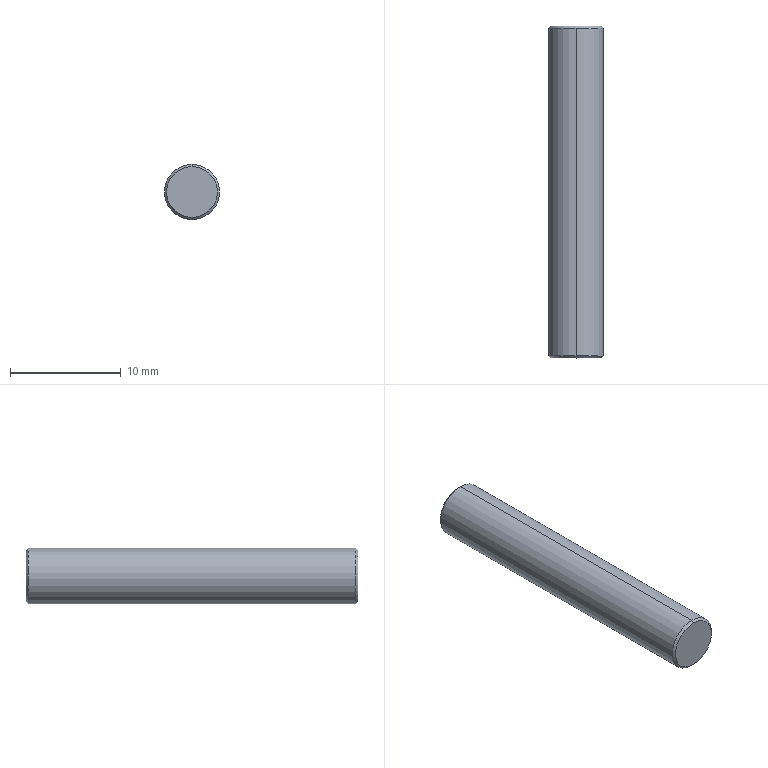Part | STEP file | 06-01-11 fibre mounting seat | 1 solid | 12 faces | box 5 x 30 x 5 mm | volume 550.393 mm3 | cone 6 | cylinder 4 | plane 2 | commonest cylinder face diameters 2.5 x2 5 x2
STEP:
#1=CARTESIAN_POINT('',(0.,22.5,-1.25));
#2=VERTEX_POINT('',#1);
#3=CARTESIAN_POINT('',(0.,22.5,1.25));
#4=VERTEX_POINT('',#3);
#5=CARTESIAN_POINT('',(0.,22.5,0.));
#6=DIRECTION('',(0.,1.,0.));
#7=DIRECTION('',(0.,0.,1.));
#8=AXIS2_PLACEMENT_3D('',#5,#6,#7);
#9=CIRCLE('',#8,1.25);
#10=EDGE_CURVE('',#2,#4,#9,.T.);
#11=ORIENTED_EDGE('',*,*,#10,.F.);
#12=CARTESIAN_POINT('',(0.,30.,-1.25));
#13=VERTEX_POINT('',#12);
#14=CARTESIAN_POINT('',(0.,30.,-1.25));
#15=DIRECTION('',(0.,1.,0.));
#16=VECTOR('',#15,1000.);
#17=LINE('',#14,#16);
#18=EDGE_CURVE('',#2,#13,#17,.T.);
#19=ORIENTED_EDGE('',*,*,#18,.T.);
#20=CARTESIAN_POINT('',(0.,30.,1.25));
#21=VERTEX_POINT('',#20);
#22=CARTESIAN_POINT('',(0.,30.,0.));
#23=DIRECTION('',(0.,1.,0.));
#24=DIRECTION('',(0.,0.,1.));
#25=AXIS2_PLACEMENT_3D('',#22,#23,#24);
#26=CIRCLE('',#25,1.25);
#27=EDGE_CURVE('',#13,#21,#26,.T.);
#28=ORIENTED_EDGE('',*,*,#27,.T.);
#29=CARTESIAN_POINT('',(0.,30.,1.25));
#30=DIRECTION('',(0.,1.,0.));
#31=VECTOR('',#30,1000.);
#32=LINE('',#29,#31);
#33=EDGE_CURVE('',#4,#21,#32,.T.);
#34=ORIENTED_EDGE('',*,*,#33,.F.);
#35=EDGE_LOOP('',(#11,#19,#28,#34));
#36=FACE_OUTER_BOUND('',#35,.T.);
#37=CARTESIAN_POINT('',(0.,30.,0.));
#38=DIRECTION('',(0.,1.,0.));
#39=DIRECTION('',(0.,0.,1.));
#40=AXIS2_PLACEMENT_3D('',#37,#38,#39);
#41=CYLINDRICAL_SURFACE('',#40,1.25);
#42=ADVANCED_FACE('',(#36),#41,.F.);
#43=CARTESIAN_POINT('',(0.,21.749,0.));
#44=VERTEX_POINT('',#43);
#45=CARTESIAN_POINT('',(0.,22.5,1.25));
#46=DIRECTION('',(0.,0.515,0.8572));
#47=VECTOR('',#46,1000.);
#48=LINE('',#45,#47);
#49=EDGE_CURVE('',#44,#4,#48,.T.);
#50=ORIENTED_EDGE('',*,*,#49,.F.);
#51=CARTESIAN_POINT('',(0.,22.5,-1.25));
#52=DIRECTION('',(0.,0.515,-0.8572));
#53=VECTOR('',#52,1000.);
#54=LINE('',#51,#53);
#55=EDGE_CURVE('',#44,#2,#54,.T.);
#56=ORIENTED_EDGE('',*,*,#55,.T.);
#57=ORIENTED_EDGE('',*,*,#10,.T.);
#58=EDGE_LOOP('',(#50,#56,#57));
#59=FACE_OUTER_BOUND('',#58,.T.);
#60=CARTESIAN_POINT('',(0.,22.5,0.));
#61=DIRECTION('',(0.,1.,0.));
#62=DIRECTION('',(0.,0.,1.));
#63=AXIS2_PLACEMENT_3D('',#60,#61,#62);
#64=CONICAL_SURFACE('',#63,1.25,1.03);
#65=ADVANCED_FACE('',(#59),#64,.F.);
#66=CARTESIAN_POINT('',(0.,30.,2.3));
#67=VERTEX_POINT('',#66);
#68=CARTESIAN_POINT('',(0.,30.,-2.3));
#69=VERTEX_POINT('',#68);
#70=CARTESIAN_POINT('',(0.,30.,0.));
#71=DIRECTION('',(0.,1.,0.));
#72=DIRECTION('',(0.,0.,1.));
#73=AXIS2_PLACEMENT_3D('',#70,#71,#72);
#74=CIRCLE('',#73,2.3);
#75=EDGE_CURVE('',#67,#69,#74,.T.);
#76=ORIENTED_EDGE('',*,*,#75,.F.);
#77=CARTESIAN_POINT('',(0.,29.8,2.5));
#78=VERTEX_POINT('',#77);
#79=CARTESIAN_POINT('',(0.,30.,2.3));
#80=DIRECTION('',(0.,-0.7071,0.7071));
#81=VECTOR('',#80,1000.);
#82=LINE('',#79,#81);
#83=EDGE_CURVE('',#67,#78,#82,.T.);
#84=ORIENTED_EDGE('',*,*,#83,.T.);
#85=CARTESIAN_POINT('',(0.,29.8,-2.5));
#86=VERTEX_POINT('',#85);
#87=CARTESIAN_POINT('',(0.,29.8,0.));
#88=DIRECTION('',(0.,-1.,0.));
#89=DIRECTION('',(0.,0.,1.));
#90=AXIS2_PLACEMENT_3D('',#87,#88,#89);
#91=CIRCLE('',#90,2.5);
#92=EDGE_CURVE('',#86,#78,#91,.T.);
#93=ORIENTED_EDGE('',*,*,#92,.F.);
#94=CARTESIAN_POINT('',(0.,30.,-2.3));
#95=DIRECTION('',(0.,-0.7071,-0.7071));
#96=VECTOR('',#95,1000.);
#97=LINE('',#94,#96);
#98=EDGE_CURVE('',#69,#86,#97,.T.);
#99=ORIENTED_EDGE('',*,*,#98,.F.);
#100=EDGE_LOOP('',(#76,#84,#93,#99));
#101=FACE_OUTER_BOUND('',#100,.T.);
#102=CARTESIAN_POINT('',(0.,30.,0.));
#103=DIRECTION('',(0.,-1.,0.));
#104=DIRECTION('',(0.,0.,-1.));
#105=AXIS2_PLACEMENT_3D('',#102,#103,#104);
#106=CONICAL_SURFACE('',#105,2.3,0.7854);
#107=ADVANCED_FACE('',(#101),#106,.T.);
#108=CARTESIAN_POINT('',(0.,0.,-2.3));
#109=VERTEX_POINT('',#108);
#110=CARTESIAN_POINT('',(0.,0.,2.3));
#111=VERTEX_POINT('',#110);
#112=CARTESIAN_POINT('',(0.,0.,0.));
#113=DIRECTION('',(0.,-1.,0.));
#114=DIRECTION('',(0.,0.,1.));
#115=AXIS2_PLACEMENT_3D('',#112,#113,#114);
#116=CIRCLE('',#115,2.3);
#117=EDGE_CURVE('',#109,#111,#116,.T.);
#118=ORIENTED_EDGE('',*,*,#117,.F.);
#119=CARTESIAN_POINT('',(0.,0.2,-2.5));
#120=VERTEX_POINT('',#119);
#121=CARTESIAN_POINT('',(0.,0.2,-2.5));
#122=DIRECTION('',(0.,0.7071,-0.7071));
#123=VECTOR('',#122,1000.);
#124=LINE('',#121,#123);
#125=EDGE_CURVE('',#109,#120,#124,.T.);
#126=ORIENTED_EDGE('',*,*,#125,.T.);
#127=CARTESIAN_POINT('',(0.,0.2,2.5));
#128=VERTEX_POINT('',#127);
#129=CARTESIAN_POINT('',(0.,0.2,0.));
#130=DIRECTION('',(0.,1.,0.));
#131=DIRECTION('',(0.,0.,1.));
#132=AXIS2_PLACEMENT_3D('',#129,#130,#131);
#133=CIRCLE('',#132,2.5);
#134=EDGE_CURVE('',#128,#120,#133,.T.);
#135=ORIENTED_EDGE('',*,*,#134,.F.);
#136=CARTESIAN_POINT('',(0.,0.2,2.5));
#137=DIRECTION('',(0.,0.7071,0.7071));
#138=VECTOR('',#137,1000.);
#139=LINE('',#136,#138);
#140=EDGE_CURVE('',#111,#128,#139,.T.);
#141=ORIENTED_EDGE('',*,*,#140,.F.);
#142=EDGE_LOOP('',(#118,#126,#135,#141));
#143=FACE_OUTER_BOUND('',#142,.T.);
#144=CARTESIAN_POINT('',(0.,0.2,0.));
#145=DIRECTION('',(0.,1.,0.));
#146=DIRECTION('',(0.,0.,1.));
#147=AXIS2_PLACEMENT_3D('',#144,#145,#146);
#148=CONICAL_SURFACE('',#147,2.5,0.7854);
#149=ADVANCED_FACE('',(#143),#148,.T.);
#150=ORIENTED_EDGE('',*,*,#92,.T.);
#151=CARTESIAN_POINT('',(0.,30.,2.5));
#152=DIRECTION('',(0.,-1.,0.));
#153=VECTOR('',#152,1000.);
#154=LINE('',#151,#153);
#155=EDGE_CURVE('',#78,#128,#154,.T.);
#156=ORIENTED_EDGE('',*,*,#155,.T.);
#157=ORIENTED_EDGE('',*,*,#134,.T.);
#158=CARTESIAN_POINT('',(0.,30.,-2.5));
#159=DIRECTION('',(0.,-1.,0.));
#160=VECTOR('',#159,1000.);
#161=LINE('',#158,#160);
#162=EDGE_CURVE('',#86,#120,#161,.T.);
#163=ORIENTED_EDGE('',*,*,#162,.F.);
#164=EDGE_LOOP('',(#150,#156,#157,#163));
#165=FACE_OUTER_BOUND('',#164,.T.);
#166=CARTESIAN_POINT('',(0.,30.,0.));
#167=DIRECTION('',(0.,-1.,0.));
#168=DIRECTION('',(0.,0.,-1.));
#169=AXIS2_PLACEMENT_3D('',#166,#167,#168);
#170=CYLINDRICAL_SURFACE('',#169,2.5);
#171=ADVANCED_FACE('',(#165),#170,.T.);
#172=ORIENTED_EDGE('',*,*,#155,.F.);
#173=CARTESIAN_POINT('',(0.,29.8,0.));
#174=DIRECTION('',(0.,-1.,0.));
#175=DIRECTION('',(0.,0.,1.));
#176=AXIS2_PLACEMENT_3D('',#173,#174,#175);
#177=CIRCLE('',#176,2.5);
#178=EDGE_CURVE('',#78,#86,#177,.T.);
#179=ORIENTED_EDGE('',*,*,#178,.T.);
#180=ORIENTED_EDGE('',*,*,#162,.T.);
#181=CARTESIAN_POINT('',(0.,0.2,0.));
#182=DIRECTION('',(0.,1.,0.));
#183=DIRECTION('',(0.,0.,1.));
#184=AXIS2_PLACEMENT_3D('',#181,#182,#183);
#185=CIRCLE('',#184,2.5);
#186=EDGE_CURVE('',#120,#128,#185,.T.);
#187=ORIENTED_EDGE('',*,*,#186,.T.);
#188=EDGE_LOOP('',(#172,#179,#180,#187));
#189=FACE_OUTER_BOUND('',#188,.T.);
#190=CARTESIAN_POINT('',(0.,30.,0.));
#191=DIRECTION('',(0.,-1.,0.));
#192=DIRECTION('',(0.,0.,-1.));
#193=AXIS2_PLACEMENT_3D('',#190,#191,#192);
#194=CYLINDRICAL_SURFACE('',#193,2.5);
#195=ADVANCED_FACE('',(#189),#194,.T.);
#196=CARTESIAN_POINT('',(0.,30.,0.));
#197=DIRECTION('',(0.,1.,0.));
#198=DIRECTION('',(0.,0.,1.));
#199=AXIS2_PLACEMENT_3D('',#196,#197,#198);
#200=CIRCLE('',#199,1.25);
#201=EDGE_CURVE('',#21,#13,#200,.T.);
#202=ORIENTED_EDGE('',*,*,#201,.F.);
#203=ORIENTED_EDGE('',*,*,#27,.F.);
#204=EDGE_LOOP('',(#202,#203));
#205=FACE_BOUND('',#204,.T.);
#206=CARTESIAN_POINT('',(0.,30.,0.));
#207=DIRECTION('',(0.,1.,0.));
#208=DIRECTION('',(0.,0.,1.));
#209=AXIS2_PLACEMENT_3D('',#206,#207,#208);
#210=CIRCLE('',#209,2.3);
#211=EDGE_CURVE('',#69,#67,#210,.T.);
#212=ORIENTED_EDGE('',*,*,#211,.T.);
#213=ORIENTED_EDGE('',*,*,#75,.T.);
#214=EDGE_LOOP('',(#212,#213));
#215=FACE_OUTER_BOUND('',#214,.T.);
#216=CARTESIAN_POINT('',(0.,30.,0.));
#217=DIRECTION('',(0.,1.,0.));
#218=DIRECTION('',(0.,0.,1.));
#219=AXIS2_PLACEMENT_3D('',#216,#217,#218);
#220=PLANE('',#219);
#221=ADVANCED_FACE('',(#205,#215),#220,.T.);
#222=CARTESIAN_POINT('',(0.,0.,0.));
#223=DIRECTION('',(0.,-1.,0.));
#224=DIRECTION('',(0.,0.,1.));
#225=AXIS2_PLACEMENT_3D('',#222,#223,#224);
#226=CIRCLE('',#225,2.3);
#227=EDGE_CURVE('',#111,#109,#226,.T.);
#228=ORIENTED_EDGE('',*,*,#227,.T.);
#229=ORIENTED_EDGE('',*,*,#117,.T.);
#230=EDGE_LOOP('',(#228,#229));
#231=FACE_OUTER_BOUND('',#230,.T.);
#232=CARTESIAN_POINT('',(0.,0.,0.));
#233=DIRECTION('',(0.,1.,0.));
#234=DIRECTION('',(0.,0.,1.));
#235=AXIS2_PLACEMENT_3D('',#232,#233,#234);
#236=PLANE('',#235);
#237=ADVANCED_FACE('',(#231),#236,.F.);
#238=ORIENTED_EDGE('',*,*,#125,.F.);
#239=ORIENTED_EDGE('',*,*,#227,.F.);
#240=ORIENTED_EDGE('',*,*,#140,.T.);
#241=ORIENTED_EDGE('',*,*,#186,.F.);
#242=EDGE_LOOP('',(#238,#239,#240,#241));
#243=FACE_OUTER_BOUND('',#242,.T.);
#244=CARTESIAN_POINT('',(0.,0.2,0.));
#245=DIRECTION('',(0.,1.,0.));
#246=DIRECTION('',(0.,0.,1.));
#247=AXIS2_PLACEMENT_3D('',#244,#245,#246);
#248=CONICAL_SURFACE('',#247,2.5,0.7854);
#249=ADVANCED_FACE('',(#243),#248,.T.);
#250=ORIENTED_EDGE('',*,*,#83,.F.);
#251=ORIENTED_EDGE('',*,*,#211,.F.);
#252=ORIENTED_EDGE('',*,*,#98,.T.);
#253=ORIENTED_EDGE('',*,*,#178,.F.);
#254=EDGE_LOOP('',(#250,#251,#252,#253));
#255=FACE_OUTER_BOUND('',#254,.T.);
#256=CARTESIAN_POINT('',(0.,30.,0.));
#257=DIRECTION('',(0.,-1.,0.));
#258=DIRECTION('',(0.,0.,-1.));
#259=AXIS2_PLACEMENT_3D('',#256,#257,#258);
#260=CONICAL_SURFACE('',#259,2.3,0.7854);
#261=ADVANCED_FACE('',(#255),#260,.T.);
#262=ORIENTED_EDGE('',*,*,#55,.F.);
#263=ORIENTED_EDGE('',*,*,#49,.T.);
#264=CARTESIAN_POINT('',(0.,22.5,0.));
#265=DIRECTION('',(0.,1.,0.));
#266=DIRECTION('',(0.,0.,1.));
#267=AXIS2_PLACEMENT_3D('',#264,#265,#266);
#268=CIRCLE('',#267,1.25);
#269=EDGE_CURVE('',#4,#2,#268,.T.);
#270=ORIENTED_EDGE('',*,*,#269,.T.);
#271=EDGE_LOOP('',(#262,#263,#270));
#272=FACE_OUTER_BOUND('',#271,.T.);
#273=CARTESIAN_POINT('',(0.,22.5,0.));
#274=DIRECTION('',(0.,1.,0.));
#275=DIRECTION('',(0.,0.,1.));
#276=AXIS2_PLACEMENT_3D('',#273,#274,#275);
#277=CONICAL_SURFACE('',#276,1.25,1.03);
#278=ADVANCED_FACE('',(#272),#277,.F.);
#279=ORIENTED_EDGE('',*,*,#18,.F.);
#280=ORIENTED_EDGE('',*,*,#269,.F.);
#281=ORIENTED_EDGE('',*,*,#33,.T.);
#282=ORIENTED_EDGE('',*,*,#201,.T.);
#283=EDGE_LOOP('',(#279,#280,#281,#282));
#284=FACE_OUTER_BOUND('',#283,.T.);
#285=CARTESIAN_POINT('',(0.,30.,0.));
#286=DIRECTION('',(0.,1.,0.));
#287=DIRECTION('',(0.,0.,1.));
#288=AXIS2_PLACEMENT_3D('',#285,#286,#287);
#289=CYLINDRICAL_SURFACE('',#288,1.25);
#290=ADVANCED_FACE('',(#284),#289,.F.);
#291=CLOSED_SHELL('',(#42,#65,#107,#149,#171,#195,#221,#237,#249,#261,#278,#290));
#292=MANIFOLD_SOLID_BREP('',#291);
#293=CARTESIAN_POINT('',(0.,0.,0.));
#294=DIRECTION('',(0.,0.,1.));
#295=DIRECTION('',(1.,0.,0.));
#296=AXIS2_PLACEMENT_3D('',#293,#294,#295);
#297=(LENGTH_UNIT()NAMED_UNIT(*)SI_UNIT(.MILLI.,.METRE.));
#298=UNCERTAINTY_MEASURE_WITH_UNIT(LENGTH_MEASURE(0.00001),#297,'','');
#299=(NAMED_UNIT(*)PLANE_ANGLE_UNIT()SI_UNIT($,.RADIAN.));
#300=(NAMED_UNIT(*)SI_UNIT($,.STERADIAN.)SOLID_ANGLE_UNIT());
#301=(GEOMETRIC_REPRESENTATION_CONTEXT(3)GLOBAL_UNCERTAINTY_ASSIGNED_CONTEXT((#298))GLOBAL_UNIT_ASSIGNED_CONTEXT((#297,#299,#300))REPRESENTATION_CONTEXT('',''));
#302=ADVANCED_BREP_SHAPE_REPRESENTATION('',(#292,#296),#301);